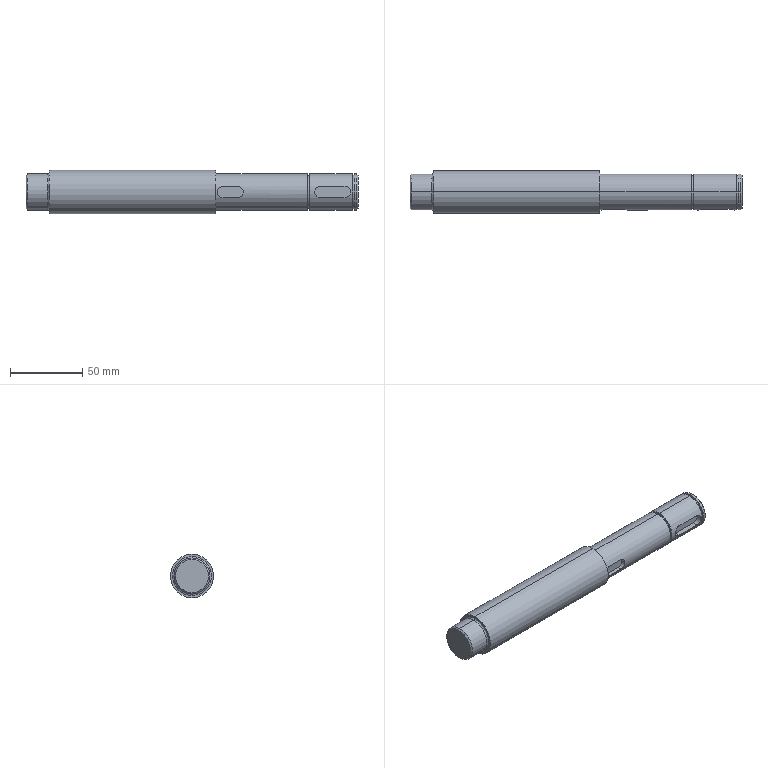Part | SolidWorks | features BaseBody 1 | 1 solid | 38 faces | box 230 x 30 x 30 mm | volume 136483 mm3 | cylinder 18 | plane 14 | cone 4 | spline 2 | commonest cylinder face diameters 25 x8 8 x4 22.5 x2 23 x2 30 x2